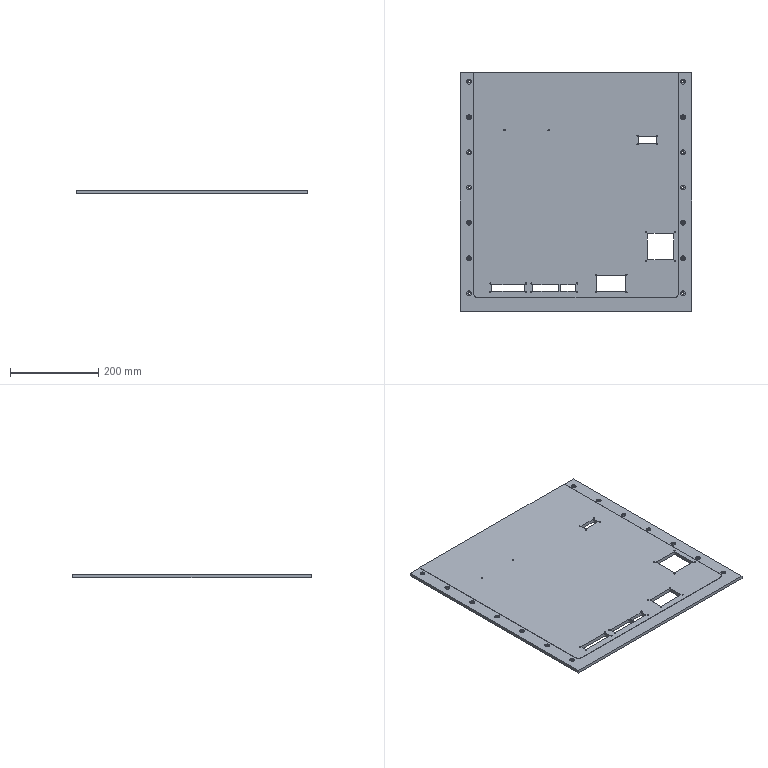Part | SolidWorks | features HoleWzd 6, MoveFace 5, BaseBody 1, Fillet 1, ICE 1 | 1 solid | 294 faces | box 525 x 540 x 8 mm | volume 2142455 mm3 | cylinder 186 | cone 60 | plane 48 | commonest cylinder face diameters 2.5 x100 5.5 x28 11 x28 2 x24 3.3 x4 18 x2